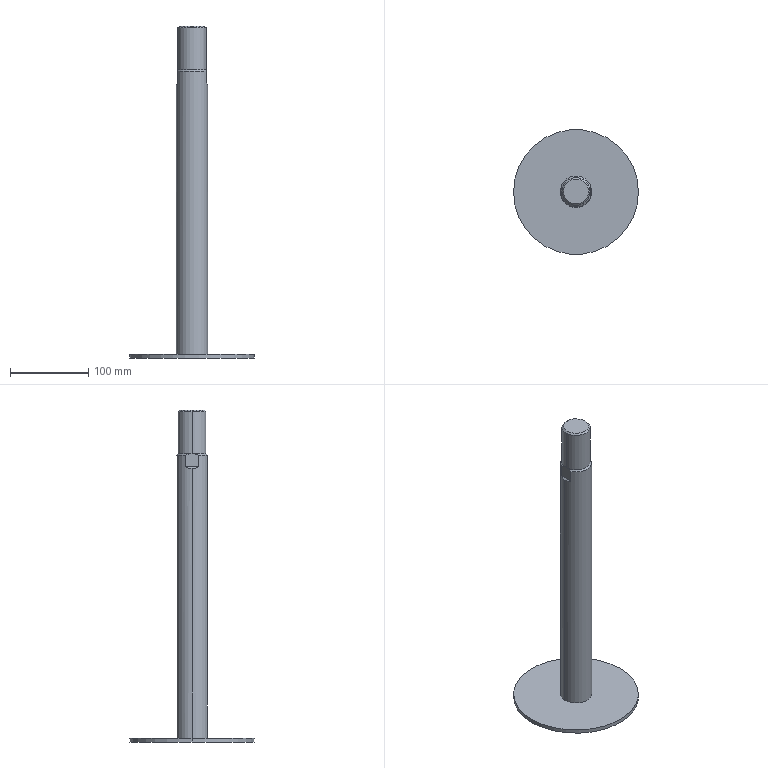Part | STEP file | CDS1FN160-250-A54Z_CS1-Rod | 1 solid | 17 faces | box 160 x 160 x 425.5 mm | volume 614336 mm3 | plane 7 | cylinder 6 | cone 4 | commonest cylinder face diameters 36 x2 40 x2 160 x2
STEP:
#1=CARTESIAN_POINT('',(0.,0.,0.));
#2=DIRECTION('',(0.,0.,1.));
#3=DIRECTION('',(1.,0.,0.));
#4=AXIS2_PLACEMENT_3D('',#1,#2,#3);
#5=CARTESIAN_POINT('',(-18.,0.,423.5));
#6=VERTEX_POINT('',#5);
#7=CARTESIAN_POINT('',(18.,0.,423.5));
#8=VERTEX_POINT('',#7);
#9=CARTESIAN_POINT('',(0.,0.,423.5));
#10=DIRECTION('',(0.,0.,-1.));
#11=DIRECTION('',(-1.,0.,0.));
#12=AXIS2_PLACEMENT_3D('',#9,#10,#11);
#13=CIRCLE('',#12,18.);
#14=CARTESIAN_POINT('',(0.,0.,0.));
#15=DIRECTION('',(0.,0.,-1.));
#16=DIRECTION('',(-1.,0.,0.));
#17=AXIS2_PLACEMENT_3D('',#14,#15,#16);
#18=CYLINDRICAL_SURFACE('',#17,18.);
#19=CARTESIAN_POINT('',(0.,-423.5));
#20=DIRECTION('',(1.,0.));
#21=VECTOR('',#20,1.);
#22=LINE('',#19,#21);
#23=(GEOMETRIC_REPRESENTATION_CONTEXT(2)PARAMETRIC_REPRESENTATION_CONTEXT()REPRESENTATION_CONTEXT('',''));
#24=DEFINITIONAL_REPRESENTATION('',(#22),#23);
#25=PCURVE('',#18,#24);
#26=CARTESIAN_POINT('',(0.,0.,425.5));
#27=DIRECTION('',(0.,0.,-1.));
#28=DIRECTION('',(-1.,0.,0.));
#29=AXIS2_PLACEMENT_3D('',#26,#27,#28);
#30=CONICAL_SURFACE('',#29,16.,0.7854);
#31=CARTESIAN_POINT('',(0.,2.));
#32=DIRECTION('',(1.,0.));
#33=VECTOR('',#32,1.);
#34=LINE('',#31,#33);
#35=(GEOMETRIC_REPRESENTATION_CONTEXT(2)PARAMETRIC_REPRESENTATION_CONTEXT()REPRESENTATION_CONTEXT('',''));
#36=DEFINITIONAL_REPRESENTATION('',(#34),#35);
#37=PCURVE('',#30,#36);
#38=SURFACE_CURVE('',#13,(#25,#37),.PCURVE_S1.);
#39=EDGE_CURVE('',#6,#8,#38,.T.);
#40=ORIENTED_EDGE('',*,*,#39,.T.);
#41=CARTESIAN_POINT('',(18.,0.,369.5));
#42=VERTEX_POINT('',#41);
#43=CARTESIAN_POINT('',(18.,0.,0.));
#44=DIRECTION('',(0.,0.,-1.));
#45=VECTOR('',#44,1.);
#46=LINE('',#43,#45);
#47=CARTESIAN_POINT('',(3.142,0.));
#48=DIRECTION('',(0.,1.));
#49=VECTOR('',#48,1.);
#50=LINE('',#47,#49);
#51=(GEOMETRIC_REPRESENTATION_CONTEXT(2)PARAMETRIC_REPRESENTATION_CONTEXT()REPRESENTATION_CONTEXT('',''));
#52=DEFINITIONAL_REPRESENTATION('',(#50),#51);
#53=PCURVE('',#18,#52);
#54=CARTESIAN_POINT('',(0.,0.,0.));
#55=DIRECTION('',(0.,0.,-1.));
#56=DIRECTION('',(-1.,0.,0.));
#57=AXIS2_PLACEMENT_3D('',#54,#55,#56);
#58=CYLINDRICAL_SURFACE('',#57,18.);
#59=CARTESIAN_POINT('',(3.142,0.));
#60=DIRECTION('',(0.,1.));
#61=VECTOR('',#60,1.);
#62=LINE('',#59,#61);
#63=(GEOMETRIC_REPRESENTATION_CONTEXT(2)PARAMETRIC_REPRESENTATION_CONTEXT()REPRESENTATION_CONTEXT('',''));
#64=DEFINITIONAL_REPRESENTATION('',(#62),#63);
#65=PCURVE('',#58,#64);
#66=SURFACE_CURVE('',#46,(#53,#65),.PCURVE_S1.);
#67=EDGE_CURVE('',#8,#42,#66,.T.);
#68=ORIENTED_EDGE('',*,*,#67,.T.);
#69=CARTESIAN_POINT('',(-18.,0.,369.5));
#70=VERTEX_POINT('',#69);
#71=CARTESIAN_POINT('',(0.,0.,369.5));
#72=DIRECTION('',(0.,0.,-1.));
#73=DIRECTION('',(-1.,0.,0.));
#74=AXIS2_PLACEMENT_3D('',#71,#72,#73);
#75=CIRCLE('',#74,18.);
#76=CARTESIAN_POINT('',(0.,-369.5));
#77=DIRECTION('',(1.,0.));
#78=VECTOR('',#77,1.);
#79=LINE('',#76,#78);
#80=(GEOMETRIC_REPRESENTATION_CONTEXT(2)PARAMETRIC_REPRESENTATION_CONTEXT()REPRESENTATION_CONTEXT('',''));
#81=DEFINITIONAL_REPRESENTATION('',(#79),#80);
#82=PCURVE('',#18,#81);
#83=CARTESIAN_POINT('',(0.,0.,369.5));
#84=DIRECTION('',(0.,0.,-1.));
#85=DIRECTION('',(-1.,0.,0.));
#86=AXIS2_PLACEMENT_3D('',#83,#84,#85);
#87=CONICAL_SURFACE('',#86,18.,0.7854);
#88=CARTESIAN_POINT('',(0.,0.));
#89=DIRECTION('',(1.,0.));
#90=VECTOR('',#89,1.);
#91=LINE('',#88,#90);
#92=(GEOMETRIC_REPRESENTATION_CONTEXT(2)PARAMETRIC_REPRESENTATION_CONTEXT()REPRESENTATION_CONTEXT('',''));
#93=DEFINITIONAL_REPRESENTATION('',(#91),#92);
#94=PCURVE('',#87,#93);
#95=SURFACE_CURVE('',#75,(#82,#94),.PCURVE_S1.);
#96=EDGE_CURVE('',#70,#42,#95,.T.);
#97=ORIENTED_EDGE('',*,*,#96,.F.);
#98=CARTESIAN_POINT('',(-18.,0.,0.));
#99=DIRECTION('',(0.,0.,-1.));
#100=VECTOR('',#99,1.);
#101=LINE('',#98,#100);
#102=CARTESIAN_POINT('',(0.,0.));
#103=DIRECTION('',(0.,1.));
#104=VECTOR('',#103,1.);
#105=LINE('',#102,#104);
#106=(GEOMETRIC_REPRESENTATION_CONTEXT(2)PARAMETRIC_REPRESENTATION_CONTEXT()REPRESENTATION_CONTEXT('',''));
#107=DEFINITIONAL_REPRESENTATION('',(#105),#106);
#108=PCURVE('',#18,#107);
#109=CARTESIAN_POINT('',(6.283,0.));
#110=DIRECTION('',(0.,1.));
#111=VECTOR('',#110,1.);
#112=LINE('',#109,#111);
#113=(GEOMETRIC_REPRESENTATION_CONTEXT(2)PARAMETRIC_REPRESENTATION_CONTEXT()REPRESENTATION_CONTEXT('',''));
#114=DEFINITIONAL_REPRESENTATION('',(#112),#113);
#115=PCURVE('',#58,#114);
#116=SURFACE_CURVE('',#101,(#108,#115),.PCURVE_S1.);
#117=EDGE_CURVE('',#6,#70,#116,.T.);
#118=ORIENTED_EDGE('',*,*,#117,.F.);
#119=EDGE_LOOP('',(#40,#68,#97,#118));
#120=FACE_BOUND('',#119,.T.);
#121=ADVANCED_FACE('',(#120),#18,.T.);
#122=CARTESIAN_POINT('',(-16.,0.,425.5));
#123=VERTEX_POINT('',#122);
#124=CARTESIAN_POINT('',(16.,0.,425.5));
#125=VERTEX_POINT('',#124);
#126=CARTESIAN_POINT('',(0.,0.,425.5));
#127=DIRECTION('',(0.,0.,-1.));
#128=DIRECTION('',(-1.,0.,0.));
#129=AXIS2_PLACEMENT_3D('',#126,#127,#128);
#130=CIRCLE('',#129,16.);
#131=CARTESIAN_POINT('',(0.,0.));
#132=DIRECTION('',(1.,0.));
#133=VECTOR('',#132,1.);
#134=LINE('',#131,#133);
#135=(GEOMETRIC_REPRESENTATION_CONTEXT(2)PARAMETRIC_REPRESENTATION_CONTEXT()REPRESENTATION_CONTEXT('',''));
#136=DEFINITIONAL_REPRESENTATION('',(#134),#135);
#137=PCURVE('',#30,#136);
#138=CARTESIAN_POINT('',(0.,0.,425.5));
#139=DIRECTION('',(0.,0.,-1.));
#140=DIRECTION('',(-1.,0.,0.));
#141=AXIS2_PLACEMENT_3D('',#138,#139,#140);
#142=PLANE('',#141);
#143=CARTESIAN_POINT('',(0.,0.));
#144=DIRECTION('',(1.,0.));
#145=AXIS2_PLACEMENT_2D('',#143,#144);
#146=CIRCLE('',#145,16.);
#147=(GEOMETRIC_REPRESENTATION_CONTEXT(2)PARAMETRIC_REPRESENTATION_CONTEXT()REPRESENTATION_CONTEXT('',''));
#148=DEFINITIONAL_REPRESENTATION('',(#146),#147);
#149=PCURVE('',#142,#148);
#150=SURFACE_CURVE('',#130,(#137,#149),.PCURVE_S1.);
#151=EDGE_CURVE('',#123,#125,#150,.T.);
#152=ORIENTED_EDGE('',*,*,#151,.T.);
#153=CARTESIAN_POINT('',(16.,0.,425.5));
#154=DIRECTION('',(0.7071,0.,-0.7071));
#155=VECTOR('',#154,1.);
#156=LINE('',#153,#155);
#157=CARTESIAN_POINT('',(3.142,0.));
#158=DIRECTION('',(0.,1.));
#159=VECTOR('',#158,1.);
#160=LINE('',#157,#159);
#161=(GEOMETRIC_REPRESENTATION_CONTEXT(2)PARAMETRIC_REPRESENTATION_CONTEXT()REPRESENTATION_CONTEXT('',''));
#162=DEFINITIONAL_REPRESENTATION('',(#160),#161);
#163=PCURVE('',#30,#162);
#164=CARTESIAN_POINT('',(0.,0.,425.5));
#165=DIRECTION('',(0.,0.,-1.));
#166=DIRECTION('',(-1.,0.,0.));
#167=AXIS2_PLACEMENT_3D('',#164,#165,#166);
#168=CONICAL_SURFACE('',#167,16.,0.7854);
#169=CARTESIAN_POINT('',(3.142,0.));
#170=DIRECTION('',(0.,1.));
#171=VECTOR('',#170,1.);
#172=LINE('',#169,#171);
#173=(GEOMETRIC_REPRESENTATION_CONTEXT(2)PARAMETRIC_REPRESENTATION_CONTEXT()REPRESENTATION_CONTEXT('',''));
#174=DEFINITIONAL_REPRESENTATION('',(#172),#173);
#175=PCURVE('',#168,#174);
#176=SURFACE_CURVE('',#156,(#163,#175),.PCURVE_S1.);
#177=EDGE_CURVE('',#125,#8,#176,.T.);
#178=ORIENTED_EDGE('',*,*,#177,.T.);
#179=ORIENTED_EDGE('',*,*,#39,.F.);
#180=CARTESIAN_POINT('',(-16.,0.,425.5));
#181=DIRECTION('',(-0.7071,0.,-0.7071));
#182=VECTOR('',#181,1.);
#183=LINE('',#180,#182);
#184=CARTESIAN_POINT('',(0.,0.));
#185=DIRECTION('',(0.,1.));
#186=VECTOR('',#185,1.);
#187=LINE('',#184,#186);
#188=(GEOMETRIC_REPRESENTATION_CONTEXT(2)PARAMETRIC_REPRESENTATION_CONTEXT()REPRESENTATION_CONTEXT('',''));
#189=DEFINITIONAL_REPRESENTATION('',(#187),#188);
#190=PCURVE('',#30,#189);
#191=CARTESIAN_POINT('',(6.283,0.));
#192=DIRECTION('',(0.,1.));
#193=VECTOR('',#192,1.);
#194=LINE('',#191,#193);
#195=(GEOMETRIC_REPRESENTATION_CONTEXT(2)PARAMETRIC_REPRESENTATION_CONTEXT()REPRESENTATION_CONTEXT('',''));
#196=DEFINITIONAL_REPRESENTATION('',(#194),#195);
#197=PCURVE('',#168,#196);
#198=SURFACE_CURVE('',#183,(#190,#197),.PCURVE_S1.);
#199=EDGE_CURVE('',#123,#6,#198,.T.);
#200=ORIENTED_EDGE('',*,*,#199,.F.);
#201=EDGE_LOOP('',(#152,#178,#179,#200));
#202=FACE_BOUND('',#201,.T.);
#203=ADVANCED_FACE('',(#202),#30,.T.);
#204=CARTESIAN_POINT('',(-80.,0.,5.));
#205=VERTEX_POINT('',#204);
#206=CARTESIAN_POINT('',(80.,0.,5.));
#207=VERTEX_POINT('',#206);
#208=CARTESIAN_POINT('',(0.,0.,5.));
#209=DIRECTION('',(0.,0.,-1.));
#210=DIRECTION('',(-1.,0.,0.));
#211=AXIS2_PLACEMENT_3D('',#208,#209,#210);
#212=CIRCLE('',#211,80.);
#213=CARTESIAN_POINT('',(0.,0.,5.));
#214=DIRECTION('',(0.,0.,-1.));
#215=DIRECTION('',(-1.,0.,0.));
#216=AXIS2_PLACEMENT_3D('',#213,#214,#215);
#217=CYLINDRICAL_SURFACE('',#216,80.);
#218=CARTESIAN_POINT('',(0.,0.));
#219=DIRECTION('',(1.,0.));
#220=VECTOR('',#219,1.);
#221=LINE('',#218,#220);
#222=(GEOMETRIC_REPRESENTATION_CONTEXT(2)PARAMETRIC_REPRESENTATION_CONTEXT()REPRESENTATION_CONTEXT('',''));
#223=DEFINITIONAL_REPRESENTATION('',(#221),#222);
#224=PCURVE('',#217,#223);
#225=CARTESIAN_POINT('',(0.,0.,5.));
#226=DIRECTION('',(0.,0.,-1.));
#227=DIRECTION('',(-1.,0.,0.));
#228=AXIS2_PLACEMENT_3D('',#225,#226,#227);
#229=PLANE('',#228);
#230=CARTESIAN_POINT('',(0.,0.));
#231=DIRECTION('',(1.,0.));
#232=AXIS2_PLACEMENT_2D('',#230,#231);
#233=CIRCLE('',#232,80.);
#234=(GEOMETRIC_REPRESENTATION_CONTEXT(2)PARAMETRIC_REPRESENTATION_CONTEXT()REPRESENTATION_CONTEXT('',''));
#235=DEFINITIONAL_REPRESENTATION('',(#233),#234);
#236=PCURVE('',#229,#235);
#237=SURFACE_CURVE('',#212,(#224,#236),.PCURVE_S1.);
#238=EDGE_CURVE('',#205,#207,#237,.T.);
#239=ORIENTED_EDGE('',*,*,#238,.T.);
#240=CARTESIAN_POINT('',(80.,0.,0.));
#241=VERTEX_POINT('',#240);
#242=CARTESIAN_POINT('',(80.,0.,5.));
#243=DIRECTION('',(0.,0.,-1.));
#244=VECTOR('',#243,1.);
#245=LINE('',#242,#244);
#246=CARTESIAN_POINT('',(3.142,0.));
#247=DIRECTION('',(0.,1.));
#248=VECTOR('',#247,1.);
#249=LINE('',#246,#248);
#250=(GEOMETRIC_REPRESENTATION_CONTEXT(2)PARAMETRIC_REPRESENTATION_CONTEXT()REPRESENTATION_CONTEXT('',''));
#251=DEFINITIONAL_REPRESENTATION('',(#249),#250);
#252=PCURVE('',#217,#251);
#253=CARTESIAN_POINT('',(0.,0.,5.));
#254=DIRECTION('',(0.,0.,-1.));
#255=DIRECTION('',(-1.,0.,0.));
#256=AXIS2_PLACEMENT_3D('',#253,#254,#255);
#257=CYLINDRICAL_SURFACE('',#256,80.);
#258=CARTESIAN_POINT('',(3.142,0.));
#259=DIRECTION('',(0.,1.));
#260=VECTOR('',#259,1.);
#261=LINE('',#258,#260);
#262=(GEOMETRIC_REPRESENTATION_CONTEXT(2)PARAMETRIC_REPRESENTATION_CONTEXT()REPRESENTATION_CONTEXT('',''));
#263=DEFINITIONAL_REPRESENTATION('',(#261),#262);
#264=PCURVE('',#257,#263);
#265=SURFACE_CURVE('',#245,(#252,#264),.PCURVE_S1.);
#266=EDGE_CURVE('',#207,#241,#265,.T.);
#267=ORIENTED_EDGE('',*,*,#266,.T.);
#268=CARTESIAN_POINT('',(-80.,0.,0.));
#269=VERTEX_POINT('',#268);
#270=CARTESIAN_POINT('',(0.,0.,0.));
#271=DIRECTION('',(0.,0.,-1.));
#272=DIRECTION('',(-1.,0.,0.));
#273=AXIS2_PLACEMENT_3D('',#270,#271,#272);
#274=CIRCLE('',#273,80.);
#275=CARTESIAN_POINT('',(0.,5.));
#276=DIRECTION('',(1.,0.));
#277=VECTOR('',#276,1.);
#278=LINE('',#275,#277);
#279=(GEOMETRIC_REPRESENTATION_CONTEXT(2)PARAMETRIC_REPRESENTATION_CONTEXT()REPRESENTATION_CONTEXT('',''));
#280=DEFINITIONAL_REPRESENTATION('',(#278),#279);
#281=PCURVE('',#217,#280);
#282=CARTESIAN_POINT('',(0.,0.,0.));
#283=DIRECTION('',(0.,0.,1.));
#284=DIRECTION('',(1.,0.,0.));
#285=AXIS2_PLACEMENT_3D('',#282,#283,#284);
#286=PLANE('',#285);
#287=CARTESIAN_POINT('',(-80.,0.));
#288=CARTESIAN_POINT('',(-80.,138.564));
#289=CARTESIAN_POINT('',(40.,69.282));
#290=CARTESIAN_POINT('',(160.,0.));
#291=CARTESIAN_POINT('',(40.,-69.282));
#292=CARTESIAN_POINT('',(-80.,-138.564));
#293=CARTESIAN_POINT('',(-80.,0.));
#294=(BOUNDED_CURVE()B_SPLINE_CURVE(2,(#287,#288,#289,#290,#291,#292,#293),.UNSPECIFIED.,.T.,.F.)B_SPLINE_CURVE_WITH_KNOTS((1,2,2,2,2,1),(-2.094,0.,2.094,4.189,6.283,8.378),.UNSPECIFIED.)CURVE()GEOMETRIC_REPRESENTATION_ITEM()RATIONAL_B_SPLINE_CURVE((1.,0.5,1.,0.5,1.,0.5,1.))REPRESENTATION_ITEM(''));
#295=(GEOMETRIC_REPRESENTATION_CONTEXT(2)PARAMETRIC_REPRESENTATION_CONTEXT()REPRESENTATION_CONTEXT('',''));
#296=DEFINITIONAL_REPRESENTATION('',(#294),#295);
#297=PCURVE('',#286,#296);
#298=SURFACE_CURVE('',#274,(#281,#297),.PCURVE_S1.);
#299=EDGE_CURVE('',#269,#241,#298,.T.);
#300=ORIENTED_EDGE('',*,*,#299,.F.);
#301=CARTESIAN_POINT('',(-80.,0.,5.));
#302=DIRECTION('',(0.,0.,-1.));
#303=VECTOR('',#302,1.);
#304=LINE('',#301,#303);
#305=CARTESIAN_POINT('',(0.,0.));
#306=DIRECTION('',(0.,1.));
#307=VECTOR('',#306,1.);
#308=LINE('',#305,#307);
#309=(GEOMETRIC_REPRESENTATION_CONTEXT(2)PARAMETRIC_REPRESENTATION_CONTEXT()REPRESENTATION_CONTEXT('',''));
#310=DEFINITIONAL_REPRESENTATION('',(#308),#309);
#311=PCURVE('',#217,#310);
#312=CARTESIAN_POINT('',(6.283,0.));
#313=DIRECTION('',(0.,1.));
#314=VECTOR('',#313,1.);
#315=LINE('',#312,#314);
#316=(GEOMETRIC_REPRESENTATION_CONTEXT(2)PARAMETRIC_REPRESENTATION_CONTEXT()REPRESENTATION_CONTEXT('',''));
#317=DEFINITIONAL_REPRESENTATION('',(#315),#316);
#318=PCURVE('',#257,#317);
#319=SURFACE_CURVE('',#304,(#311,#318),.PCURVE_S1.);
#320=EDGE_CURVE('',#205,#269,#319,.T.);
#321=ORIENTED_EDGE('',*,*,#320,.F.);
#322=EDGE_LOOP('',(#239,#267,#300,#321));
#323=FACE_BOUND('',#322,.T.);
#324=ADVANCED_FACE('',(#323),#217,.T.);
#325=CARTESIAN_POINT('',(18.,8.718,352.5));
#326=VERTEX_POINT('',#325);
#327=CARTESIAN_POINT('',(20.,0.,350.5));
#328=VERTEX_POINT('',#327);
#329=CARTESIAN_POINT('',(18.,8.718,352.5));
#330=CARTESIAN_POINT('',(19.322,5.988,351.178));
#331=CARTESIAN_POINT('',(20.,3.033,350.5));
#332=CARTESIAN_POINT('',(20.,0.,350.5));
#333=(BOUNDED_CURVE()B_SPLINE_CURVE(3,(#329,#330,#331,#332),.UNSPECIFIED.,.F.,.F.)B_SPLINE_CURVE_WITH_KNOTS((4,4),(5.832,6.283),.PIECEWISE_BEZIER_KNOTS.)CURVE()GEOMETRIC_REPRESENTATION_ITEM()RATIONAL_B_SPLINE_CURVE((1.,0.9831,0.9831,1.))REPRESENTATION_ITEM(''));
#334=CARTESIAN_POINT('',(0.,0.,482.069));
#335=DIRECTION('',(0.,0.,-1.));
#336=DIRECTION('',(-1.,0.,0.));
#337=AXIS2_PLACEMENT_3D('',#334,#335,#336);
#338=CYLINDRICAL_SURFACE('',#337,20.);
#339=CARTESIAN_POINT('',(2.691,129.569));
#340=CARTESIAN_POINT('',(2.697,129.628));
#341=CARTESIAN_POINT('',(2.711,129.743));
#342=CARTESIAN_POINT('',(2.731,129.91));
#343=CARTESIAN_POINT('',(2.752,130.069));
#344=CARTESIAN_POINT('',(2.772,130.221));
#345=CARTESIAN_POINT('',(2.793,130.365));
#346=CARTESIAN_POINT('',(2.813,130.501));
#347=CARTESIAN_POINT('',(2.834,130.63));
#348=CARTESIAN_POINT('',(2.854,130.75));
#349=CARTESIAN_POINT('',(2.875,130.863));
#350=CARTESIAN_POINT('',(2.895,130.967));
#351=CARTESIAN_POINT('',(2.916,131.064));
#352=CARTESIAN_POINT('',(2.937,131.151));
#353=CARTESIAN_POINT('',(2.957,131.231));
#354=CARTESIAN_POINT('',(2.978,131.302));
#355=CARTESIAN_POINT('',(2.998,131.365));
#356=CARTESIAN_POINT('',(3.019,131.42));
#357=CARTESIAN_POINT('',(3.039,131.466));
#358=CARTESIAN_POINT('',(3.06,131.503));
#359=CARTESIAN_POINT('',(3.08,131.533));
#360=CARTESIAN_POINT('',(3.101,131.553));
#361=CARTESIAN_POINT('',(3.121,131.566));
#362=CARTESIAN_POINT('',(3.135,131.569));
#363=CARTESIAN_POINT('',(3.142,131.569));
#364=B_SPLINE_CURVE_WITH_KNOTS('',3,(#339,#340,#341,#342,#343,#344,#345,#346,#347,#348,#349,#350,#351,#352,#353,#354,#355,#356,#357,#358,#359,#360,#361,#362,#363),.UNSPECIFIED.,.F.,.F.,(4,1,1,1,1,1,1,1,1,1,1,1,1,1,1,1,1,1,1,1,1,1,4),(5.832,5.853,5.873,5.894,5.914,5.935,5.955,5.976,5.996,6.017,6.037,6.058,6.078,6.099,6.119,6.14,6.16,6.181,6.201,6.222,6.242,6.263,6.283),.QUASI_UNIFORM_KNOTS.);
#365=(GEOMETRIC_REPRESENTATION_CONTEXT(2)PARAMETRIC_REPRESENTATION_CONTEXT()REPRESENTATION_CONTEXT('',''));
#366=DEFINITIONAL_REPRESENTATION('',(#364),#365);
#367=PCURVE('',#338,#366);
#368=CARTESIAN_POINT('',(20.,-80.,350.5));
#369=DIRECTION('',(-0.7071,0.,-0.7071));
#370=DIRECTION('',(-0.7071,0.,0.7071));
#371=AXIS2_PLACEMENT_3D('',#368,#369,#370);
#372=PLANE('',#371);
#373=CARTESIAN_POINT('',(2.828,88.718));
#374=CARTESIAN_POINT('',(0.959,85.988));
#375=CARTESIAN_POINT('',(0.,83.033));
#376=CARTESIAN_POINT('',(0.,80.));
#377=(BOUNDED_CURVE()B_SPLINE_CURVE(3,(#373,#374,#375,#376),.UNSPECIFIED.,.F.,.F.)B_SPLINE_CURVE_WITH_KNOTS((4,4),(5.832,6.283),.PIECEWISE_BEZIER_KNOTS.)CURVE()GEOMETRIC_REPRESENTATION_ITEM()RATIONAL_B_SPLINE_CURVE((1.,0.9831,0.9831,1.))REPRESENTATION_ITEM(''));
#378=(GEOMETRIC_REPRESENTATION_CONTEXT(2)PARAMETRIC_REPRESENTATION_CONTEXT()REPRESENTATION_CONTEXT('',''));
#379=DEFINITIONAL_REPRESENTATION('',(#377),#378);
#380=PCURVE('',#372,#379);
#381=SURFACE_CURVE('',#333,(#367,#380),.PCURVE_S1.);
#382=EDGE_CURVE('',#326,#328,#381,.T.);
#383=ORIENTED_EDGE('',*,*,#382,.T.);
#384=CARTESIAN_POINT('',(20.,0.,5.));
#385=VERTEX_POINT('',#384);
#386=CARTESIAN_POINT('',(20.,0.,482.069));
#387=DIRECTION('',(0.,0.,-1.));
#388=VECTOR('',#387,1.);
#389=LINE('',#386,#388);
#390=CARTESIAN_POINT('',(3.142,0.));
#391=DIRECTION('',(0.,1.));
#392=VECTOR('',#391,1.);
#393=LINE('',#390,#392);
#394=(GEOMETRIC_REPRESENTATION_CONTEXT(2)PARAMETRIC_REPRESENTATION_CONTEXT()REPRESENTATION_CONTEXT('',''));
#395=DEFINITIONAL_REPRESENTATION('',(#393),#394);
#396=PCURVE('',#338,#395);
#397=CARTESIAN_POINT('',(0.,0.,482.069));
#398=DIRECTION('',(0.,0.,-1.));
#399=DIRECTION('',(-1.,0.,0.));
#400=AXIS2_PLACEMENT_3D('',#397,#398,#399);
#401=CYLINDRICAL_SURFACE('',#400,20.);
#402=CARTESIAN_POINT('',(3.142,0.));
#403=DIRECTION('',(0.,1.));
#404=VECTOR('',#403,1.);
#405=LINE('',#402,#404);
#406=(GEOMETRIC_REPRESENTATION_CONTEXT(2)PARAMETRIC_REPRESENTATION_CONTEXT()REPRESENTATION_CONTEXT('',''));
#407=DEFINITIONAL_REPRESENTATION('',(#405),#406);
#408=PCURVE('',#401,#407);
#409=SURFACE_CURVE('',#389,(#396,#408),.PCURVE_S1.);
#410=EDGE_CURVE('',#328,#385,#409,.T.);
#411=ORIENTED_EDGE('',*,*,#410,.T.);
#412=CARTESIAN_POINT('',(-20.,0.,5.));
#413=VERTEX_POINT('',#412);
#414=CARTESIAN_POINT('',(0.,0.,5.));
#415=DIRECTION('',(0.,0.,-1.));
#416=DIRECTION('',(-1.,0.,0.));
#417=AXIS2_PLACEMENT_3D('',#414,#415,#416);
#418=CIRCLE('',#417,20.);
#419=CARTESIAN_POINT('',(0.,477.069));
#420=DIRECTION('',(1.,0.));
#421=VECTOR('',#420,1.);
#422=LINE('',#419,#421);
#423=(GEOMETRIC_REPRESENTATION_CONTEXT(2)PARAMETRIC_REPRESENTATION_CONTEXT()REPRESENTATION_CONTEXT('',''));
#424=DEFINITIONAL_REPRESENTATION('',(#422),#423);
#425=PCURVE('',#338,#424);
#426=CARTESIAN_POINT('',(0.,0.));
#427=DIRECTION('',(1.,0.));
#428=AXIS2_PLACEMENT_2D('',#426,#427);
#429=CIRCLE('',#428,20.);
#430=(GEOMETRIC_REPRESENTATION_CONTEXT(2)PARAMETRIC_REPRESENTATION_CONTEXT()REPRESENTATION_CONTEXT('',''));
#431=DEFINITIONAL_REPRESENTATION('',(#429),#430);
#432=PCURVE('',#229,#431);
#433=SURFACE_CURVE('',#418,(#425,#432),.PCURVE_S1.);
#434=EDGE_CURVE('',#413,#385,#433,.T.);
#435=ORIENTED_EDGE('',*,*,#434,.F.);
#436=CARTESIAN_POINT('',(-20.,0.,350.5));
#437=VERTEX_POINT('',#436);
#438=CARTESIAN_POINT('',(-20.,0.,482.069));
#439=DIRECTION('',(0.,0.,-1.));
#440=VECTOR('',#439,1.);
#441=LINE('',#438,#440);
#442=CARTESIAN_POINT('',(0.,0.));
#443=DIRECTION('',(0.,1.));
#444=VECTOR('',#443,1.);
#445=LINE('',#442,#444);
#446=(GEOMETRIC_REPRESENTATION_CONTEXT(2)PARAMETRIC_REPRESENTATION_CONTEXT()REPRESENTATION_CONTEXT('',''));
#447=DEFINITIONAL_REPRESENTATION('',(#445),#446);
#448=PCURVE('',#338,#447);
#449=CARTESIAN_POINT('',(6.283,0.));
#450=DIRECTION('',(0.,1.));
#451=VECTOR('',#450,1.);
#452=LINE('',#449,#451);
#453=(GEOMETRIC_REPRESENTATION_CONTEXT(2)PARAMETRIC_REPRESENTATION_CONTEXT()REPRESENTATION_CONTEXT('',''));
#454=DEFINITIONAL_REPRESENTATION('',(#452),#453);
#455=PCURVE('',#401,#454);
#456=SURFACE_CURVE('',#441,(#448,#455),.PCURVE_S1.);
#457=EDGE_CURVE('',#437,#413,#456,.T.);
#458=ORIENTED_EDGE('',*,*,#457,.F.);
#459=CARTESIAN_POINT('',(-18.,8.718,352.5));
#460=VERTEX_POINT('',#459);
#461=CARTESIAN_POINT('',(-20.,0.,350.5));
#462=CARTESIAN_POINT('',(-20.,3.033,350.5));
#463=CARTESIAN_POINT('',(-19.322,5.988,351.178));
#464=CARTESIAN_POINT('',(-18.,8.718,352.5));
#465=(BOUNDED_CURVE()B_SPLINE_CURVE(3,(#461,#462,#463,#464),.UNSPECIFIED.,.F.,.F.)B_SPLINE_CURVE_WITH_KNOTS((4,4),(0.,0.451),.PIECEWISE_BEZIER_KNOTS.)CURVE()GEOMETRIC_REPRESENTATION_ITEM()RATIONAL_B_SPLINE_CURVE((1.,0.9831,0.9831,1.))REPRESENTATION_ITEM(''));
#466=CARTESIAN_POINT('',(0.,131.569));
#467=CARTESIAN_POINT('',(0.006776,131.569));
#468=CARTESIAN_POINT('',(0.02034,131.566));
#469=CARTESIAN_POINT('',(0.04074,131.553));
#470=CARTESIAN_POINT('',(0.06117,131.533));
#471=CARTESIAN_POINT('',(0.08164,131.503));
#472=CARTESIAN_POINT('',(0.1021,131.466));
#473=CARTESIAN_POINT('',(0.1227,131.42));
#474=CARTESIAN_POINT('',(0.1432,131.365));
#475=CARTESIAN_POINT('',(0.1638,131.302));
#476=CARTESIAN_POINT('',(0.1843,131.231));
#477=CARTESIAN_POINT('',(0.2049,131.151));
#478=CARTESIAN_POINT('',(0.2255,131.064));
#479=CARTESIAN_POINT('',(0.2461,130.967));
#480=CARTESIAN_POINT('',(0.2667,130.863));
#481=CARTESIAN_POINT('',(0.2873,130.75));
#482=CARTESIAN_POINT('',(0.3078,130.63));
#483=CARTESIAN_POINT('',(0.3284,130.501));
#484=CARTESIAN_POINT('',(0.3489,130.365));
#485=CARTESIAN_POINT('',(0.3694,130.221));
#486=CARTESIAN_POINT('',(0.3899,130.069));
#487=CARTESIAN_POINT('',(0.4103,129.91));
#488=CARTESIAN_POINT('',(0.4307,129.743));
#489=CARTESIAN_POINT('',(0.4443,129.628));
#490=CARTESIAN_POINT('',(0.451,129.569));
#491=B_SPLINE_CURVE_WITH_KNOTS('',3,(#466,#467,#468,#469,#470,#471,#472,#473,#474,#475,#476,#477,#478,#479,#480,#481,#482,#483,#484,#485,#486,#487,#488,#489,#490),.UNSPECIFIED.,.F.,.F.,(4,1,1,1,1,1,1,1,1,1,1,1,1,1,1,1,1,1,1,1,1,1,4),(0.,0.0205,0.041,0.0615,0.082,0.1025,0.123,0.1435,0.164,0.1845,0.205,0.2255,0.246,0.2665,0.287,0.3075,0.328,0.3485,0.369,0.3895,0.41,0.4305,0.451),.QUASI_UNIFORM_KNOTS.);
#492=(GEOMETRIC_REPRESENTATION_CONTEXT(2)PARAMETRIC_REPRESENTATION_CONTEXT()REPRESENTATION_CONTEXT('',''));
#493=DEFINITIONAL_REPRESENTATION('',(#491),#492);
#494=PCURVE('',#338,#493);
#495=CARTESIAN_POINT('',(-20.,-80.,350.5));
#496=DIRECTION('',(0.7071,0.,-0.7071));
#497=DIRECTION('',(-0.7071,0.,-0.7071));
#498=AXIS2_PLACEMENT_3D('',#495,#496,#497);
#499=PLANE('',#498);
#500=CARTESIAN_POINT('',(0.,80.));
#501=CARTESIAN_POINT('',(0.,83.033));
#502=CARTESIAN_POINT('',(-0.959,85.988));
#503=CARTESIAN_POINT('',(-2.828,88.718));
#504=(BOUNDED_CURVE()B_SPLINE_CURVE(3,(#500,#501,#502,#503),.UNSPECIFIED.,.F.,.F.)B_SPLINE_CURVE_WITH_KNOTS((4,4),(0.,0.451),.PIECEWISE_BEZIER_KNOTS.)CURVE()GEOMETRIC_REPRESENTATION_ITEM()RATIONAL_B_SPLINE_CURVE((1.,0.9831,0.9831,1.))REPRESENTATION_ITEM(''));
#505=(GEOMETRIC_REPRESENTATION_CONTEXT(2)PARAMETRIC_REPRESENTATION_CONTEXT()REPRESENTATION_CONTEXT('',''));
#506=DEFINITIONAL_REPRESENTATION('',(#504),#505);
#507=PCURVE('',#499,#506);
#508=SURFACE_CURVE('',#465,(#494,#507),.PCURVE_S1.);
#509=EDGE_CURVE('',#437,#460,#508,.T.);
#510=ORIENTED_EDGE('',*,*,#509,.T.);
#511=CARTESIAN_POINT('',(-18.,8.718,367.5));
#512=VERTEX_POINT('',#511);
#513=CARTESIAN_POINT('',(-18.,8.718,482.069));
#514=DIRECTION('',(0.,0.,1.));
#515=VECTOR('',#514,1.);
#516=LINE('',#513,#515);
#517=CARTESIAN_POINT('',(0.451,0.));
#518=DIRECTION('',(0.,-1.));
#519=VECTOR('',#518,1.);
#520=LINE('',#517,#519);
#521=(GEOMETRIC_REPRESENTATION_CONTEXT(2)PARAMETRIC_REPRESENTATION_CONTEXT()REPRESENTATION_CONTEXT('',''));
#522=DEFINITIONAL_REPRESENTATION('',(#520),#521);
#523=PCURVE('',#338,#522);
#524=CARTESIAN_POINT('',(-18.,-80.,352.5));
#525=DIRECTION('',(1.,0.,0.));
#526=DIRECTION('',(0.,0.,-1.));
#527=AXIS2_PLACEMENT_3D('',#524,#525,#526);
#528=PLANE('',#527);
#529=CARTESIAN_POINT('',(-129.569,88.718));
#530=DIRECTION('',(-1.,0.));
#531=VECTOR('',#530,1.);
#532=LINE('',#529,#531);
#533=(GEOMETRIC_REPRESENTATION_CONTEXT(2)PARAMETRIC_REPRESENTATION_CONTEXT()REPRESENTATION_CONTEXT('',''));
#534=DEFINITIONAL_REPRESENTATION('',(#532),#533);
#535=PCURVE('',#528,#534);
#536=SURFACE_CURVE('',#516,(#523,#535),.PCURVE_S1.);
#537=EDGE_CURVE('',#460,#512,#536,.T.);
#538=ORIENTED_EDGE('',*,*,#537,.T.);
#539=CARTESIAN_POINT('',(18.,8.718,367.5));
#540=VERTEX_POINT('',#539);
#541=CARTESIAN_POINT('',(0.,0.,367.5));
#542=DIRECTION('',(0.,0.,-1.));
#543=DIRECTION('',(-1.,0.,0.));
#544=AXIS2_PLACEMENT_3D('',#541,#542,#543);
#545=CIRCLE('',#544,20.);
#546=CARTESIAN_POINT('',(0.,114.569));
#547=DIRECTION('',(1.,0.));
#548=VECTOR('',#547,1.);
#549=LINE('',#546,#548);
#550=(GEOMETRIC_REPRESENTATION_CONTEXT(2)PARAMETRIC_REPRESENTATION_CONTEXT()REPRESENTATION_CONTEXT('',''));
#551=DEFINITIONAL_REPRESENTATION('',(#549),#550);
#552=PCURVE('',#338,#551);
#553=CARTESIAN_POINT('',(0.,2.));
#554=DIRECTION('',(1.,0.));
#555=VECTOR('',#554,1.);
#556=LINE('',#553,#555);
#557=(GEOMETRIC_REPRESENTATION_CONTEXT(2)PARAMETRIC_REPRESENTATION_CONTEXT()REPRESENTATION_CONTEXT('',''));
#558=DEFINITIONAL_REPRESENTATION('',(#556),#557);
#559=PCURVE('',#87,#558);
#560=SURFACE_CURVE('',#545,(#552,#559),.PCURVE_S1.);
#561=EDGE_CURVE('',#512,#540,#560,.T.);
#562=ORIENTED_EDGE('',*,*,#561,.T.);
#563=CARTESIAN_POINT('',(18.,8.718,482.069));
#564=DIRECTION('',(0.,0.,-1.));
#565=VECTOR('',#564,1.);
#566=LINE('',#563,#565);
#567=CARTESIAN_POINT('',(2.691,0.));
#568=DIRECTION('',(0.,1.));
#569=VECTOR('',#568,1.);
#570=LINE('',#567,#569);
#571=(GEOMETRIC_REPRESENTATION_CONTEXT(2)PARAMETRIC_REPRESENTATION_CONTEXT()REPRESENTATION_CONTEXT('',''));
#572=DEFINITIONAL_REPRESENTATION('',(#570),#571);
#573=PCURVE('',#338,#572);
#574=CARTESIAN_POINT('',(18.,-80.,352.5));
#575=DIRECTION('',(-1.,0.,0.));
#576=DIRECTION('',(0.,0.,1.));
#577=AXIS2_PLACEMENT_3D('',#574,#575,#576);
#578=PLANE('',#577);
#579=CARTESIAN_POINT('',(129.569,88.718));
#580=DIRECTION('',(-1.,0.));
#581=VECTOR('',#580,1.);
#582=LINE('',#579,#581);
#583=(GEOMETRIC_REPRESENTATION_CONTEXT(2)PARAMETRIC_REPRESENTATION_CONTEXT()REPRESENTATION_CONTEXT('',''));
#584=DEFINITIONAL_REPRESENTATION('',(#582),#583);
#585=PCURVE('',#578,#584);
#586=SURFACE_CURVE('',#566,(#573,#585),.PCURVE_S1.);
#587=EDGE_CURVE('',#540,#326,#586,.T.);
#588=ORIENTED_EDGE('',*,*,#587,.T.);
#589=EDGE_LOOP('',(#383,#411,#435,#458,#510,#538,#562,#588));
#590=FACE_BOUND('',#589,.T.);
#591=ADVANCED_FACE('',(#590),#338,.T.);
#592=ORIENTED_EDGE('',*,*,#561,.F.);
#593=CARTESIAN_POINT('',(-18.,8.718,367.5));
#594=CARTESIAN_POINT('',(-18.,8.033,367.799));
#595=CARTESIAN_POINT('',(-18.,7.333,368.075));
#596=CARTESIAN_POINT('',(-18.,5.906,368.568));
#597=CARTESIAN_POINT('',(-18.,5.187,368.781));
#598=CARTESIAN_POINT('',(-18.,3.732,369.131));
#599=CARTESIAN_POINT('',(-18.,2.997,369.267));
#600=CARTESIAN_POINT('',(-18.,1.883,369.406));
#601=CARTESIAN_POINT('',(-18.,1.509,369.441));
#602=CARTESIAN_POINT('',(-18.,0.7572,369.488));
#603=CARTESIAN_POINT('',(-18.,0.3777,369.5));
#604=CARTESIAN_POINT('',(-18.,0.,369.5));
#605=B_SPLINE_CURVE_WITH_KNOTS('',3,(#593,#594,#595,#596,#597,#598,#599,#600,#601,#602,#603,#604),.UNSPECIFIED.,.F.,.F.,(4,2,2,2,2,4),(0.01306,0.01529,0.01752,0.01975,0.02086,0.02197),.UNSPECIFIED.);
#606=CARTESIAN_POINT('',(0.451,2.));
#607=CARTESIAN_POINT('',(0.4454,1.946));
#608=CARTESIAN_POINT('',(0.4341,1.839));
#609=CARTESIAN_POINT('',(0.4167,1.683));
#610=CARTESIAN_POINT('',(0.3988,1.532));
#611=CARTESIAN_POINT('',(0.3806,1.386));
#612=CARTESIAN_POINT('',(0.362,1.246));
#613=CARTESIAN_POINT('',(0.3429,1.111));
#614=CARTESIAN_POINT('',(0.3235,0.9835));
#615=CARTESIAN_POINT('',(0.3038,0.8626));
#616=CARTESIAN_POINT('',(0.2838,0.7487));
#617=CARTESIAN_POINT('',(0.2635,0.6421));
#618=CARTESIAN_POINT('',(0.2429,0.5429));
#619=CARTESIAN_POINT('',(0.222,0.4513));
#620=CARTESIAN_POINT('',(0.2008,0.3676));
#621=CARTESIAN_POINT('',(0.1793,0.2919));
#622=CARTESIAN_POINT('',(0.1576,0.2245));
#623=CARTESIAN_POINT('',(0.1357,0.1654));
#624=CARTESIAN_POINT('',(0.1135,0.1151));
#625=CARTESIAN_POINT('',(0.09113,0.07346));
#626=CARTESIAN_POINT('',(0.06856,0.04083));
#627=CARTESIAN_POINT('',(0.04582,0.01734));
#628=CARTESIAN_POINT('',(0.02292,0.003165));
#629=CARTESIAN_POINT('',(0.007631,-0.000006235));
#630=CARTESIAN_POINT('',(0.,0.));
#631=B_SPLINE_CURVE_WITH_KNOTS('',3,(#606,#607,#608,#609,#610,#611,#612,#613,#614,#615,#616,#617,#618,#619,#620,#621,#622,#623,#624,#625,#626,#627,#628,#629,#630),.UNSPECIFIED.,.F.,.F.,(4,1,1,1,1,1,1,1,1,1,1,1,1,1,1,1,1,1,1,1,1,1,4),(0.01306,0.01347,0.01387,0.01428,0.01468,0.01509,0.01549,0.0159,0.0163,0.01671,0.01711,0.01752,0.01792,0.01833,0.01873,0.01914,0.01954,0.01995,0.02035,0.02076,0.02116,0.02157,0.02197),.QUASI_UNIFORM_KNOTS.);
#632=(GEOMETRIC_REPRESENTATION_CONTEXT(2)PARAMETRIC_REPRESENTATION_CONTEXT()REPRESENTATION_CONTEXT('',''));
#633=DEFINITIONAL_REPRESENTATION('',(#631),#632);
#634=PCURVE('',#87,#633);
#635=CARTESIAN_POINT('',(-15.,88.718));
#636=CARTESIAN_POINT('',(-15.299,88.033));
#637=CARTESIAN_POINT('',(-15.575,87.333));
#638=CARTESIAN_POINT('',(-16.068,85.906));
#639=CARTESIAN_POINT('',(-16.281,85.187));
#640=CARTESIAN_POINT('',(-16.631,83.732));
#641=CARTESIAN_POINT('',(-16.767,82.997));
#642=CARTESIAN_POINT('',(-16.906,81.883));
#643=CARTESIAN_POINT('',(-16.941,81.509));
#644=CARTESIAN_POINT('',(-16.988,80.757));
#645=CARTESIAN_POINT('',(-17.,80.378));
#646=CARTESIAN_POINT('',(-17.,80.));
#647=B_SPLINE_CURVE_WITH_KNOTS('',3,(#635,#636,#637,#638,#639,#640,#641,#642,#643,#644,#645,#646),.UNSPECIFIED.,.F.,.F.,(4,2,2,2,2,4),(0.01306,0.01529,0.01752,0.01975,0.02086,0.02197),.UNSPECIFIED.);
#648=(GEOMETRIC_REPRESENTATION_CONTEXT(2)PARAMETRIC_REPRESENTATION_CONTEXT()REPRESENTATION_CONTEXT('',''));
#649=DEFINITIONAL_REPRESENTATION('',(#647),#648);
#650=PCURVE('',#528,#649);
#651=SURFACE_CURVE('',#605,(#634,#650),.PCURVE_S1.);
#652=EDGE_CURVE('',#512,#70,#651,.T.);
#653=ORIENTED_EDGE('',*,*,#652,.T.);
#654=ORIENTED_EDGE('',*,*,#96,.T.);
#655=CARTESIAN_POINT('',(18.,0.,369.5));
#656=CARTESIAN_POINT('',(18.,0.3777,369.5));
#657=CARTESIAN_POINT('',(18.,0.7572,369.488));
#658=CARTESIAN_POINT('',(18.,1.509,369.441));
#659=CARTESIAN_POINT('',(18.,1.883,369.406));
#660=CARTESIAN_POINT('',(18.,2.997,369.267));
#661=CARTESIAN_POINT('',(18.,3.732,369.131));
#662=CARTESIAN_POINT('',(18.,5.187,368.781));
#663=CARTESIAN_POINT('',(18.,5.906,368.568));
#664=CARTESIAN_POINT('',(18.,7.333,368.075));
#665=CARTESIAN_POINT('',(18.,8.033,367.799));
#666=CARTESIAN_POINT('',(18.,8.718,367.5));
#667=B_SPLINE_CURVE_WITH_KNOTS('',3,(#655,#656,#657,#658,#659,#660,#661,#662,#663,#664,#665,#666),.UNSPECIFIED.,.F.,.F.,(4,2,2,2,2,4),(0.01468,0.0158,0.01692,0.01916,0.0214,0.02364),.UNSPECIFIED.);
#668=CARTESIAN_POINT('',(3.142,0.));
#669=CARTESIAN_POINT('',(3.134,-0.000006235));
#670=CARTESIAN_POINT('',(3.119,0.003165));
#671=CARTESIAN_POINT('',(3.096,0.01734));
#672=CARTESIAN_POINT('',(3.073,0.04083));
#673=CARTESIAN_POINT('',(3.05,0.07346));
#674=CARTESIAN_POINT('',(3.028,0.1151));
#675=CARTESIAN_POINT('',(3.006,0.1654));
#676=CARTESIAN_POINT('',(2.984,0.2245));
#677=CARTESIAN_POINT('',(2.962,0.2919));
#678=CARTESIAN_POINT('',(2.941,0.3676));
#679=CARTESIAN_POINT('',(2.92,0.4513));
#680=CARTESIAN_POINT('',(2.899,0.5429));
#681=CARTESIAN_POINT('',(2.878,0.6421));
#682=CARTESIAN_POINT('',(2.858,0.7487));
#683=CARTESIAN_POINT('',(2.838,0.8626));
#684=CARTESIAN_POINT('',(2.818,0.9835));
#685=CARTESIAN_POINT('',(2.799,1.111));
#686=CARTESIAN_POINT('',(2.78,1.246));
#687=CARTESIAN_POINT('',(2.761,1.386));
#688=CARTESIAN_POINT('',(2.743,1.532));
#689=CARTESIAN_POINT('',(2.725,1.683));
#690=CARTESIAN_POINT('',(2.708,1.839));
#691=CARTESIAN_POINT('',(2.696,1.946));
#692=CARTESIAN_POINT('',(2.691,2.));
#693=B_SPLINE_CURVE_WITH_KNOTS('',3,(#668,#669,#670,#671,#672,#673,#674,#675,#676,#677,#678,#679,#680,#681,#682,#683,#684,#685,#686,#687,#688,#689,#690,#691,#692),.UNSPECIFIED.,.F.,.F.,(4,1,1,1,1,1,1,1,1,1,1,1,1,1,1,1,1,1,1,1,1,1,4),(0.01468,0.01508,0.01549,0.0159,0.0163,0.01671,0.01712,0.01753,0.01793,0.01834,0.01875,0.01916,0.01956,0.01997,0.02038,0.02078,0.02119,0.0216,0.02201,0.02241,0.02282,0.02323,0.02364),.QUASI_UNIFORM_KNOTS.);
#694=(GEOMETRIC_REPRESENTATION_CONTEXT(2)PARAMETRIC_REPRESENTATION_CONTEXT()REPRESENTATION_CONTEXT('',''));
#695=DEFINITIONAL_REPRESENTATION('',(#693),#694);
#696=PCURVE('',#87,#695);
#697=CARTESIAN_POINT('',(17.,80.));
#698=CARTESIAN_POINT('',(17.,80.378));
#699=CARTESIAN_POINT('',(16.988,80.757));
#700=CARTESIAN_POINT('',(16.941,81.509));
#701=CARTESIAN_POINT('',(16.906,81.883));
#702=CARTESIAN_POINT('',(16.767,82.997));
#703=CARTESIAN_POINT('',(16.631,83.732));
#704=CARTESIAN_POINT('',(16.281,85.187));
#705=CARTESIAN_POINT('',(16.068,85.906));
#706=CARTESIAN_POINT('',(15.575,87.333));
#707=CARTESIAN_POINT('',(15.299,88.033));
#708=CARTESIAN_POINT('',(15.,88.718));
#709=B_SPLINE_CURVE_WITH_KNOTS('',3,(#697,#698,#699,#700,#701,#702,#703,#704,#705,#706,#707,#708),.UNSPECIFIED.,.F.,.F.,(4,2,2,2,2,4),(0.01468,0.0158,0.01692,0.01916,0.0214,0.02364),.UNSPECIFIED.);
#710=(GEOMETRIC_REPRESENTATION_CONTEXT(2)PARAMETRIC_REPRESENTATION_CONTEXT()REPRESENTATION_CONTEXT('',''));
#711=DEFINITIONAL_REPRESENTATION('',(#709),#710);
#712=PCURVE('',#578,#711);
#713=SURFACE_CURVE('',#667,(#696,#712),.PCURVE_S1.);
#714=EDGE_CURVE('',#42,#540,#713,.T.);
#715=ORIENTED_EDGE('',*,*,#714,.T.);
#716=EDGE_LOOP('',(#592,#653,#654,#715));
#717=FACE_BOUND('',#716,.T.);
#718=ADVANCED_FACE('',(#717),#87,.T.);
#719=ORIENTED_EDGE('',*,*,#410,.F.);
#720=CARTESIAN_POINT('',(18.,-8.718,352.5));
#721=VERTEX_POINT('',#720);
#722=CARTESIAN_POINT('',(20.,0.,350.5));
#723=CARTESIAN_POINT('',(20.,-3.033,350.5));
#724=CARTESIAN_POINT('',(19.322,-5.988,351.178));
#725=CARTESIAN_POINT('',(18.,-8.718,352.5));
#726=(BOUNDED_CURVE()B_SPLINE_CURVE(3,(#722,#723,#724,#725),.UNSPECIFIED.,.F.,.F.)B_SPLINE_CURVE_WITH_KNOTS((4,4),(0.,0.451),.PIECEWISE_BEZIER_KNOTS.)CURVE()GEOMETRIC_REPRESENTATION_ITEM()RATIONAL_B_SPLINE_CURVE((1.,0.9831,0.9831,1.))REPRESENTATION_ITEM(''));
#727=CARTESIAN_POINT('',(3.142,131.569));
#728=CARTESIAN_POINT('',(3.148,131.569));
#729=CARTESIAN_POINT('',(3.162,131.566));
#730=CARTESIAN_POINT('',(3.182,131.553));
#731=CARTESIAN_POINT('',(3.203,131.533));
#732=CARTESIAN_POINT('',(3.223,131.503));
#733=CARTESIAN_POINT('',(3.244,131.466));
#734=CARTESIAN_POINT('',(3.264,131.42));
#735=CARTESIAN_POINT('',(3.285,131.365));
#736=CARTESIAN_POINT('',(3.305,131.302));
#737=CARTESIAN_POINT('',(3.326,131.231));
#738=CARTESIAN_POINT('',(3.347,131.151));
#739=CARTESIAN_POINT('',(3.367,131.064));
#740=CARTESIAN_POINT('',(3.388,130.967));
#741=CARTESIAN_POINT('',(3.408,130.863));
#742=CARTESIAN_POINT('',(3.429,130.75));
#743=CARTESIAN_POINT('',(3.449,130.63));
#744=CARTESIAN_POINT('',(3.47,130.501));
#745=CARTESIAN_POINT('',(3.49,130.365));
#746=CARTESIAN_POINT('',(3.511,130.221));
#747=CARTESIAN_POINT('',(3.531,130.069));
#748=CARTESIAN_POINT('',(3.552,129.91));
#749=CARTESIAN_POINT('',(3.572,129.743));
#750=CARTESIAN_POINT('',(3.586,129.628));
#751=CARTESIAN_POINT('',(3.593,129.569));
#752=B_SPLINE_CURVE_WITH_KNOTS('',3,(#727,#728,#729,#730,#731,#732,#733,#734,#735,#736,#737,#738,#739,#740,#741,#742,#743,#744,#745,#746,#747,#748,#749,#750,#751),.UNSPECIFIED.,.F.,.F.,(4,1,1,1,1,1,1,1,1,1,1,1,1,1,1,1,1,1,1,1,1,1,4),(0.,0.0205,0.041,0.0615,0.082,0.1025,0.123,0.1435,0.164,0.1845,0.205,0.2255,0.246,0.2665,0.287,0.3075,0.328,0.3485,0.369,0.3895,0.41,0.4305,0.451),.QUASI_UNIFORM_KNOTS.);
#753=(GEOMETRIC_REPRESENTATION_CONTEXT(2)PARAMETRIC_REPRESENTATION_CONTEXT()REPRESENTATION_CONTEXT('',''));
#754=DEFINITIONAL_REPRESENTATION('',(#752),#753);
#755=PCURVE('',#401,#754);
#756=CARTESIAN_POINT('',(0.,80.));
#757=CARTESIAN_POINT('',(0.,76.967));
#758=CARTESIAN_POINT('',(0.959,74.012));
#759=CARTESIAN_POINT('',(2.828,71.282));
#760=(BOUNDED_CURVE()B_SPLINE_CURVE(3,(#756,#757,#758,#759),.UNSPECIFIED.,.F.,.F.)B_SPLINE_CURVE_WITH_KNOTS((4,4),(0.,0.451),.PIECEWISE_BEZIER_KNOTS.)CURVE()GEOMETRIC_REPRESENTATION_ITEM()RATIONAL_B_SPLINE_CURVE((1.,0.9831,0.9831,1.))REPRESENTATION_ITEM(''));
#761=(GEOMETRIC_REPRESENTATION_CONTEXT(2)PARAMETRIC_REPRESENTATION_CONTEXT()REPRESENTATION_CONTEXT('',''));
#762=DEFINITIONAL_REPRESENTATION('',(#760),#761);
#763=PCURVE('',#372,#762);
#764=SURFACE_CURVE('',#726,(#755,#763),.PCURVE_S1.);
#765=EDGE_CURVE('',#328,#721,#764,.T.);
#766=ORIENTED_EDGE('',*,*,#765,.T.);
#767=CARTESIAN_POINT('',(18.,-8.718,367.5));
#768=VERTEX_POINT('',#767);
#769=CARTESIAN_POINT('',(18.,-8.718,482.069));
#770=DIRECTION('',(0.,0.,1.));
#771=VECTOR('',#770,1.);
#772=LINE('',#769,#771);
#773=CARTESIAN_POINT('',(3.593,0.));
#774=DIRECTION('',(0.,-1.));
#775=VECTOR('',#774,1.);
#776=LINE('',#773,#775);
#777=(GEOMETRIC_REPRESENTATION_CONTEXT(2)PARAMETRIC_REPRESENTATION_CONTEXT()REPRESENTATION_CONTEXT('',''));
#778=DEFINITIONAL_REPRESENTATION('',(#776),#777);
#779=PCURVE('',#401,#778);
#780=CARTESIAN_POINT('',(129.569,71.282));
#781=DIRECTION('',(1.,0.));
#782=VECTOR('',#781,1.);
#783=LINE('',#780,#782);
#784=(GEOMETRIC_REPRESENTATION_CONTEXT(2)PARAMETRIC_REPRESENTATION_CONTEXT()REPRESENTATION_CONTEXT('',''));
#785=DEFINITIONAL_REPRESENTATION('',(#783),#784);
#786=PCURVE('',#578,#785);
#787=SURFACE_CURVE('',#772,(#779,#786),.PCURVE_S1.);
#788=EDGE_CURVE('',#721,#768,#787,.T.);
#789=ORIENTED_EDGE('',*,*,#788,.T.);
#790=CARTESIAN_POINT('',(-18.,-8.718,367.5));
#791=VERTEX_POINT('',#790);
#792=CARTESIAN_POINT('',(0.,0.,367.5));
#793=DIRECTION('',(0.,0.,-1.));
#794=DIRECTION('',(-1.,0.,0.));
#795=AXIS2_PLACEMENT_3D('',#792,#793,#794);
#796=CIRCLE('',#795,20.);
#797=CARTESIAN_POINT('',(0.,114.569));
#798=DIRECTION('',(1.,0.));
#799=VECTOR('',#798,1.);
#800=LINE('',#797,#799);
#801=(GEOMETRIC_REPRESENTATION_CONTEXT(2)PARAMETRIC_REPRESENTATION_CONTEXT()REPRESENTATION_CONTEXT('',''));
#802=DEFINITIONAL_REPRESENTATION('',(#800),#801);
#803=PCURVE('',#401,#802);
#804=CARTESIAN_POINT('',(0.,0.,369.5));
#805=DIRECTION('',(0.,0.,-1.));
#806=DIRECTION('',(-1.,0.,0.));
#807=AXIS2_PLACEMENT_3D('',#804,#805,#806);
#808=CONICAL_SURFACE('',#807,18.,0.7854);
#809=CARTESIAN_POINT('',(0.,2.));
#810=DIRECTION('',(1.,0.));
#811=VECTOR('',#810,1.);
#812=LINE('',#809,#811);
#813=(GEOMETRIC_REPRESENTATION_CONTEXT(2)PARAMETRIC_REPRESENTATION_CONTEXT()REPRESENTATION_CONTEXT('',''));
#814=DEFINITIONAL_REPRESENTATION('',(#812),#813);
#815=PCURVE('',#808,#814);
#816=SURFACE_CURVE('',#796,(#803,#815),.PCURVE_S1.);
#817=EDGE_CURVE('',#768,#791,#816,.T.);
#818=ORIENTED_EDGE('',*,*,#817,.T.);
#819=CARTESIAN_POINT('',(-18.,-8.718,352.5));
#820=VERTEX_POINT('',#819);
#821=CARTESIAN_POINT('',(-18.,-8.718,482.069));
#822=DIRECTION('',(0.,0.,-1.));
#823=VECTOR('',#822,1.);
#824=LINE('',#821,#823);
#825=CARTESIAN_POINT('',(5.832,0.));
#826=DIRECTION('',(0.,1.));
#827=VECTOR('',#826,1.);
#828=LINE('',#825,#827);
#829=(GEOMETRIC_REPRESENTATION_CONTEXT(2)PARAMETRIC_REPRESENTATION_CONTEXT()REPRESENTATION_CONTEXT('',''));
#830=DEFINITIONAL_REPRESENTATION('',(#828),#829);
#831=PCURVE('',#401,#830);
#832=CARTESIAN_POINT('',(-129.569,71.282));
#833=DIRECTION('',(1.,0.));
#834=VECTOR('',#833,1.);
#835=LINE('',#832,#834);
#836=(GEOMETRIC_REPRESENTATION_CONTEXT(2)PARAMETRIC_REPRESENTATION_CONTEXT()REPRESENTATION_CONTEXT('',''));
#837=DEFINITIONAL_REPRESENTATION('',(#835),#836);
#838=PCURVE('',#528,#837);
#839=SURFACE_CURVE('',#824,(#831,#838),.PCURVE_S1.);
#840=EDGE_CURVE('',#791,#820,#839,.T.);
#841=ORIENTED_EDGE('',*,*,#840,.T.);
#842=CARTESIAN_POINT('',(-18.,-8.718,352.5));
#843=CARTESIAN_POINT('',(-19.322,-5.988,351.178));
#844=CARTESIAN_POINT('',(-20.,-3.033,350.5));
#845=CARTESIAN_POINT('',(-20.,0.,350.5));
#846=(BOUNDED_CURVE()B_SPLINE_CURVE(3,(#842,#843,#844,#845),.UNSPECIFIED.,.F.,.F.)B_SPLINE_CURVE_WITH_KNOTS((4,4),(5.832,6.283),.PIECEWISE_BEZIER_KNOTS.)CURVE()GEOMETRIC_REPRESENTATION_ITEM()RATIONAL_B_SPLINE_CURVE((1.,0.9831,0.9831,1.))REPRESENTATION_ITEM(''));
#847=CARTESIAN_POINT('',(5.832,129.569));
#848=CARTESIAN_POINT('',(5.839,129.628));
#849=CARTESIAN_POINT('',(5.853,129.743));
#850=CARTESIAN_POINT('',(5.873,129.91));
#851=CARTESIAN_POINT('',(5.893,130.069));
#852=CARTESIAN_POINT('',(5.914,130.221));
#853=CARTESIAN_POINT('',(5.934,130.365));
#854=CARTESIAN_POINT('',(5.955,130.501));
#855=CARTESIAN_POINT('',(5.975,130.63));
#856=CARTESIAN_POINT('',(5.996,130.75));
#857=CARTESIAN_POINT('',(6.016,130.863));
#858=CARTESIAN_POINT('',(6.037,130.967));
#859=CARTESIAN_POINT('',(6.058,131.064));
#860=CARTESIAN_POINT('',(6.078,131.151));
#861=CARTESIAN_POINT('',(6.099,131.231));
#862=CARTESIAN_POINT('',(6.119,131.302));
#863=CARTESIAN_POINT('',(6.14,131.365));
#864=CARTESIAN_POINT('',(6.161,131.42));
#865=CARTESIAN_POINT('',(6.181,131.466));
#866=CARTESIAN_POINT('',(6.202,131.503));
#867=CARTESIAN_POINT('',(6.222,131.533));
#868=CARTESIAN_POINT('',(6.242,131.553));
#869=CARTESIAN_POINT('',(6.263,131.566));
#870=CARTESIAN_POINT('',(6.276,131.569));
#871=CARTESIAN_POINT('',(6.283,131.569));
#872=B_SPLINE_CURVE_WITH_KNOTS('',3,(#847,#848,#849,#850,#851,#852,#853,#854,#855,#856,#857,#858,#859,#860,#861,#862,#863,#864,#865,#866,#867,#868,#869,#870,#871),.UNSPECIFIED.,.F.,.F.,(4,1,1,1,1,1,1,1,1,1,1,1,1,1,1,1,1,1,1,1,1,1,4),(5.832,5.853,5.873,5.894,5.914,5.935,5.955,5.976,5.996,6.017,6.037,6.058,6.078,6.099,6.119,6.14,6.16,6.181,6.201,6.222,6.242,6.263,6.283),.QUASI_UNIFORM_KNOTS.);
#873=(GEOMETRIC_REPRESENTATION_CONTEXT(2)PARAMETRIC_REPRESENTATION_CONTEXT()REPRESENTATION_CONTEXT('',''));
#874=DEFINITIONAL_REPRESENTATION('',(#872),#873);
#875=PCURVE('',#401,#874);
#876=CARTESIAN_POINT('',(-2.828,71.282));
#877=CARTESIAN_POINT('',(-0.959,74.012));
#878=CARTESIAN_POINT('',(0.,76.967));
#879=CARTESIAN_POINT('',(0.,80.));
#880=(BOUNDED_CURVE()B_SPLINE_CURVE(3,(#876,#877,#878,#879),.UNSPECIFIED.,.F.,.F.)B_SPLINE_CURVE_WITH_KNOTS((4,4),(5.832,6.283),.PIECEWISE_BEZIER_KNOTS.)CURVE()GEOMETRIC_REPRESENTATION_ITEM()RATIONAL_B_SPLINE_CURVE((1.,0.9831,0.9831,1.))REPRESENTATION_ITEM(''));
#881=(GEOMETRIC_REPRESENTATION_CONTEXT(2)PARAMETRIC_REPRESENTATION_CONTEXT()REPRESENTATION_CONTEXT('',''));
#882=DEFINITIONAL_REPRESENTATION('',(#880),#881);
#883=PCURVE('',#499,#882);
#884=SURFACE_CURVE('',#846,(#875,#883),.PCURVE_S1.);
#885=EDGE_CURVE('',#820,#437,#884,.T.);
#886=ORIENTED_EDGE('',*,*,#885,.T.);
#887=ORIENTED_EDGE('',*,*,#457,.T.);
#888=CARTESIAN_POINT('',(0.,0.,5.));
#889=DIRECTION('',(0.,0.,-1.));
#890=DIRECTION('',(-1.,0.,0.));
#891=AXIS2_PLACEMENT_3D('',#888,#889,#890);
#892=CIRCLE('',#891,20.);
#893=CARTESIAN_POINT('',(0.,477.069));
#894=DIRECTION('',(1.,0.));
#895=VECTOR('',#894,1.);
#896=LINE('',#893,#895);
#897=(GEOMETRIC_REPRESENTATION_CONTEXT(2)PARAMETRIC_REPRESENTATION_CONTEXT()REPRESENTATION_CONTEXT('',''));
#898=DEFINITIONAL_REPRESENTATION('',(#896),#897);
#899=PCURVE('',#401,#898);
#900=CARTESIAN_POINT('',(0.,0.));
#901=DIRECTION('',(1.,0.));
#902=AXIS2_PLACEMENT_2D('',#900,#901);
#903=CIRCLE('',#902,20.);
#904=(GEOMETRIC_REPRESENTATION_CONTEXT(2)PARAMETRIC_REPRESENTATION_CONTEXT()REPRESENTATION_CONTEXT('',''));
#905=DEFINITIONAL_REPRESENTATION('',(#903),#904);
#906=PCURVE('',#229,#905);
#907=SURFACE_CURVE('',#892,(#899,#906),.PCURVE_S1.);
#908=EDGE_CURVE('',#385,#413,#907,.T.);
#909=ORIENTED_EDGE('',*,*,#908,.F.);
#910=EDGE_LOOP('',(#719,#766,#789,#818,#841,#886,#887,#909));
#911=FACE_BOUND('',#910,.T.);
#912=ADVANCED_FACE('',(#911),#401,.T.);
#913=ORIENTED_EDGE('',*,*,#238,.F.);
#914=CARTESIAN_POINT('',(0.,0.,5.));
#915=DIRECTION('',(0.,0.,-1.));
#916=DIRECTION('',(-1.,0.,0.));
#917=AXIS2_PLACEMENT_3D('',#914,#915,#916);
#918=CIRCLE('',#917,80.);
#919=CARTESIAN_POINT('',(0.,0.));
#920=DIRECTION('',(1.,0.));
#921=AXIS2_PLACEMENT_2D('',#919,#920);
#922=CIRCLE('',#921,80.);
#923=(GEOMETRIC_REPRESENTATION_CONTEXT(2)PARAMETRIC_REPRESENTATION_CONTEXT()REPRESENTATION_CONTEXT('',''));
#924=DEFINITIONAL_REPRESENTATION('',(#922),#923);
#925=PCURVE('',#229,#924);
#926=CARTESIAN_POINT('',(0.,0.));
#927=DIRECTION('',(1.,0.));
#928=VECTOR('',#927,1.);
#929=LINE('',#926,#928);
#930=(GEOMETRIC_REPRESENTATION_CONTEXT(2)PARAMETRIC_REPRESENTATION_CONTEXT()REPRESENTATION_CONTEXT('',''));
#931=DEFINITIONAL_REPRESENTATION('',(#929),#930);
#932=PCURVE('',#257,#931);
#933=SURFACE_CURVE('',#918,(#925,#932),.PCURVE_S1.);
#934=EDGE_CURVE('',#207,#205,#933,.T.);
#935=ORIENTED_EDGE('',*,*,#934,.F.);
#936=EDGE_LOOP('',(#913,#935));
#937=FACE_BOUND('',#936,.T.);
#938=ORIENTED_EDGE('',*,*,#434,.T.);
#939=ORIENTED_EDGE('',*,*,#908,.T.);
#940=EDGE_LOOP('',(#938,#939));
#941=FACE_BOUND('',#940,.T.);
#942=ADVANCED_FACE('',(#937,#941),#229,.F.);
#943=ORIENTED_EDGE('',*,*,#266,.F.);
#944=ORIENTED_EDGE('',*,*,#934,.T.);
#945=ORIENTED_EDGE('',*,*,#320,.T.);
#946=CARTESIAN_POINT('',(0.,0.,0.));
#947=DIRECTION('',(0.,0.,-1.));
#948=DIRECTION('',(-1.,0.,0.));
#949=AXIS2_PLACEMENT_3D('',#946,#947,#948);
#950=CIRCLE('',#949,80.);
#951=CARTESIAN_POINT('',(0.,5.));
#952=DIRECTION('',(1.,0.));
#953=VECTOR('',#952,1.);
#954=LINE('',#951,#953);
#955=(GEOMETRIC_REPRESENTATION_CONTEXT(2)PARAMETRIC_REPRESENTATION_CONTEXT()REPRESENTATION_CONTEXT('',''));
#956=DEFINITIONAL_REPRESENTATION('',(#954),#955);
#957=PCURVE('',#257,#956);
#958=CARTESIAN_POINT('',(-80.,0.));
#959=CARTESIAN_POINT('',(-80.,138.564));
#960=CARTESIAN_POINT('',(40.,69.282));
#961=CARTESIAN_POINT('',(160.,0.));
#962=CARTESIAN_POINT('',(40.,-69.282));
#963=CARTESIAN_POINT('',(-80.,-138.564));
#964=CARTESIAN_POINT('',(-80.,0.));
#965=(BOUNDED_CURVE()B_SPLINE_CURVE(2,(#958,#959,#960,#961,#962,#963,#964),.UNSPECIFIED.,.T.,.F.)B_SPLINE_CURVE_WITH_KNOTS((1,2,2,2,2,1),(-2.094,0.,2.094,4.189,6.283,8.378),.UNSPECIFIED.)CURVE()GEOMETRIC_REPRESENTATION_ITEM()RATIONAL_B_SPLINE_CURVE((1.,0.5,1.,0.5,1.,0.5,1.))REPRESENTATION_ITEM(''));
#966=(GEOMETRIC_REPRESENTATION_CONTEXT(2)PARAMETRIC_REPRESENTATION_CONTEXT()REPRESENTATION_CONTEXT('',''));
#967=DEFINITIONAL_REPRESENTATION('',(#965),#966);
#968=PCURVE('',#286,#967);
#969=SURFACE_CURVE('',#950,(#957,#968),.PCURVE_S1.);
#970=EDGE_CURVE('',#241,#269,#969,.T.);
#971=ORIENTED_EDGE('',*,*,#970,.F.);
#972=EDGE_LOOP('',(#943,#944,#945,#971));
#973=FACE_BOUND('',#972,.T.);
#974=ADVANCED_FACE('',(#973),#257,.T.);
#975=ORIENTED_EDGE('',*,*,#299,.T.);
#976=ORIENTED_EDGE('',*,*,#970,.T.);
#977=EDGE_LOOP('',(#975,#976));
#978=FACE_BOUND('',#977,.T.);
#979=ADVANCED_FACE('',(#978),#286,.F.);
#980=ORIENTED_EDGE('',*,*,#177,.F.);
#981=CARTESIAN_POINT('',(0.,0.,425.5));
#982=DIRECTION('',(0.,0.,-1.));
#983=DIRECTION('',(-1.,0.,0.));
#984=AXIS2_PLACEMENT_3D('',#981,#982,#983);
#985=CIRCLE('',#984,16.);
#986=CARTESIAN_POINT('',(0.,0.));
#987=DIRECTION('',(1.,0.));
#988=VECTOR('',#987,1.);
#989=LINE('',#986,#988);
#990=(GEOMETRIC_REPRESENTATION_CONTEXT(2)PARAMETRIC_REPRESENTATION_CONTEXT()REPRESENTATION_CONTEXT('',''));
#991=DEFINITIONAL_REPRESENTATION('',(#989),#990);
#992=PCURVE('',#168,#991);
#993=CARTESIAN_POINT('',(0.,0.));
#994=DIRECTION('',(1.,0.));
#995=AXIS2_PLACEMENT_2D('',#993,#994);
#996=CIRCLE('',#995,16.);
#997=(GEOMETRIC_REPRESENTATION_CONTEXT(2)PARAMETRIC_REPRESENTATION_CONTEXT()REPRESENTATION_CONTEXT('',''));
#998=DEFINITIONAL_REPRESENTATION('',(#996),#997);
#999=PCURVE('',#142,#998);
#1000=SURFACE_CURVE('',#985,(#992,#999),.PCURVE_S1.);
#1001=EDGE_CURVE('',#125,#123,#1000,.T.);
#1002=ORIENTED_EDGE('',*,*,#1001,.T.);
#1003=ORIENTED_EDGE('',*,*,#199,.T.);
#1004=CARTESIAN_POINT('',(0.,0.,423.5));
#1005=DIRECTION('',(0.,0.,-1.));
#1006=DIRECTION('',(-1.,0.,0.));
#1007=AXIS2_PLACEMENT_3D('',#1004,#1005,#1006);
#1008=CIRCLE('',#1007,18.);
#1009=CARTESIAN_POINT('',(0.,2.));
#1010=DIRECTION('',(1.,0.));
#1011=VECTOR('',#1010,1.);
#1012=LINE('',#1009,#1011);
#1013=(GEOMETRIC_REPRESENTATION_CONTEXT(2)PARAMETRIC_REPRESENTATION_CONTEXT()REPRESENTATION_CONTEXT('',''));
#1014=DEFINITIONAL_REPRESENTATION('',(#1012),#1013);
#1015=PCURVE('',#168,#1014);
#1016=CARTESIAN_POINT('',(0.,-423.5));
#1017=DIRECTION('',(1.,0.));
#1018=VECTOR('',#1017,1.);
#1019=LINE('',#1016,#1018);
#1020=(GEOMETRIC_REPRESENTATION_CONTEXT(2)PARAMETRIC_REPRESENTATION_CONTEXT()REPRESENTATION_CONTEXT('',''));
#1021=DEFINITIONAL_REPRESENTATION('',(#1019),#1020);
#1022=PCURVE('',#58,#1021);
#1023=SURFACE_CURVE('',#1008,(#1015,#1022),.PCURVE_S1.);
#1024=EDGE_CURVE('',#8,#6,#1023,.T.);
#1025=ORIENTED_EDGE('',*,*,#1024,.F.);
#1026=EDGE_LOOP('',(#980,#1002,#1003,#1025));
#1027=FACE_BOUND('',#1026,.T.);
#1028=ADVANCED_FACE('',(#1027),#168,.T.);
#1029=ORIENTED_EDGE('',*,*,#67,.F.);
#1030=ORIENTED_EDGE('',*,*,#1024,.T.);
#1031=ORIENTED_EDGE('',*,*,#117,.T.);
#1032=CARTESIAN_POINT('',(0.,0.,369.5));
#1033=DIRECTION('',(0.,0.,-1.));
#1034=DIRECTION('',(-1.,0.,0.));
#1035=AXIS2_PLACEMENT_3D('',#1032,#1033,#1034);
#1036=CIRCLE('',#1035,18.);
#1037=CARTESIAN_POINT('',(0.,-369.5));
#1038=DIRECTION('',(1.,0.));
#1039=VECTOR('',#1038,1.);
#1040=LINE('',#1037,#1039);
#1041=(GEOMETRIC_REPRESENTATION_CONTEXT(2)PARAMETRIC_REPRESENTATION_CONTEXT()REPRESENTATION_CONTEXT('',''));
#1042=DEFINITIONAL_REPRESENTATION('',(#1040),#1041);
#1043=PCURVE('',#58,#1042);
#1044=CARTESIAN_POINT('',(0.,0.));
#1045=DIRECTION('',(1.,0.));
#1046=VECTOR('',#1045,1.);
#1047=LINE('',#1044,#1046);
#1048=(GEOMETRIC_REPRESENTATION_CONTEXT(2)PARAMETRIC_REPRESENTATION_CONTEXT()REPRESENTATION_CONTEXT('',''));
#1049=DEFINITIONAL_REPRESENTATION('',(#1047),#1048);
#1050=PCURVE('',#808,#1049);
#1051=SURFACE_CURVE('',#1036,(#1043,#1050),.PCURVE_S1.);
#1052=EDGE_CURVE('',#42,#70,#1051,.T.);
#1053=ORIENTED_EDGE('',*,*,#1052,.F.);
#1054=EDGE_LOOP('',(#1029,#1030,#1031,#1053));
#1055=FACE_BOUND('',#1054,.T.);
#1056=ADVANCED_FACE('',(#1055),#58,.T.);
#1057=ORIENTED_EDGE('',*,*,#1052,.T.);
#1058=CARTESIAN_POINT('',(-18.,0.,369.5));
#1059=CARTESIAN_POINT('',(-18.,-1.51,369.5));
#1060=CARTESIAN_POINT('',(-18.,-2.996,369.308));
#1061=CARTESIAN_POINT('',(-18.,-4.828,368.867));
#1062=CARTESIAN_POINT('',(-18.,-5.194,368.769));
#1063=CARTESIAN_POINT('',(-18.,-5.917,368.555));
#1064=CARTESIAN_POINT('',(-18.,-6.275,368.44));
#1065=CARTESIAN_POINT('',(-18.,-7.338,368.073));
#1066=CARTESIAN_POINT('',(-18.,-8.033,367.798));
#1067=CARTESIAN_POINT('',(-18.,-8.718,367.5));
#1068=B_SPLINE_CURVE_WITH_KNOTS('',3,(#1058,#1059,#1060,#1061,#1062,#1063,#1064,#1065,#1066,#1067),.UNSPECIFIED.,.F.,.F.,(4,2,2,2,4),(0.02197,0.02643,0.02754,0.02865,0.03088),.UNSPECIFIED.);
#1069=CARTESIAN_POINT('',(6.283,0.));
#1070=CARTESIAN_POINT('',(6.276,-0.000000513));
#1071=CARTESIAN_POINT('',(6.26,0.00316));
#1072=CARTESIAN_POINT('',(6.238,0.01726));
#1073=CARTESIAN_POINT('',(6.215,0.0406));
#1074=CARTESIAN_POINT('',(6.192,0.07306));
#1075=CARTESIAN_POINT('',(6.17,0.1145));
#1076=CARTESIAN_POINT('',(6.148,0.1648));
#1077=CARTESIAN_POINT('',(6.126,0.2237));
#1078=CARTESIAN_POINT('',(6.104,0.2912));
#1079=CARTESIAN_POINT('',(6.083,0.3671));
#1080=CARTESIAN_POINT('',(6.061,0.4513));
#1081=CARTESIAN_POINT('',(6.04,0.5435));
#1082=CARTESIAN_POINT('',(6.019,0.6436));
#1083=CARTESIAN_POINT('',(5.999,0.7514));
#1084=CARTESIAN_POINT('',(5.979,0.8661));
#1085=CARTESIAN_POINT('',(5.959,0.9874));
#1086=CARTESIAN_POINT('',(5.94,1.115));
#1087=CARTESIAN_POINT('',(5.921,1.249));
#1088=CARTESIAN_POINT('',(5.902,1.388));
#1089=CARTESIAN_POINT('',(5.884,1.533));
#1090=CARTESIAN_POINT('',(5.866,1.683));
#1091=CARTESIAN_POINT('',(5.849,1.839));
#1092=CARTESIAN_POINT('',(5.838,1.946));
#1093=CARTESIAN_POINT('',(5.832,2.));
#1094=B_SPLINE_CURVE_WITH_KNOTS('',3,(#1069,#1070,#1071,#1072,#1073,#1074,#1075,#1076,#1077,#1078,#1079,#1080,#1081,#1082,#1083,#1084,#1085,#1086,#1087,#1088,#1089,#1090,#1091,#1092,#1093),.UNSPECIFIED.,.F.,.F.,(4,1,1,1,1,1,1,1,1,1,1,1,1,1,1,1,1,1,1,1,1,1,4),(0.02197,0.02238,0.02278,0.02319,0.02359,0.024,0.0244,0.02481,0.02521,0.02562,0.02602,0.02643,0.02683,0.02724,0.02764,0.02805,0.02845,0.02886,0.02926,0.02966,0.03007,0.03047,0.03088),.QUASI_UNIFORM_KNOTS.);
#1095=(GEOMETRIC_REPRESENTATION_CONTEXT(2)PARAMETRIC_REPRESENTATION_CONTEXT()REPRESENTATION_CONTEXT('',''));
#1096=DEFINITIONAL_REPRESENTATION('',(#1094),#1095);
#1097=PCURVE('',#808,#1096);
#1098=CARTESIAN_POINT('',(-17.,80.));
#1099=CARTESIAN_POINT('',(-17.,78.49));
#1100=CARTESIAN_POINT('',(-16.808,77.004));
#1101=CARTESIAN_POINT('',(-16.367,75.172));
#1102=CARTESIAN_POINT('',(-16.269,74.806));
#1103=CARTESIAN_POINT('',(-16.055,74.083));
#1104=CARTESIAN_POINT('',(-15.94,73.725));
#1105=CARTESIAN_POINT('',(-15.573,72.662));
#1106=CARTESIAN_POINT('',(-15.298,71.967));
#1107=CARTESIAN_POINT('',(-15.,71.282));
#1108=B_SPLINE_CURVE_WITH_KNOTS('',3,(#1098,#1099,#1100,#1101,#1102,#1103,#1104,#1105,#1106,#1107),.UNSPECIFIED.,.F.,.F.,(4,2,2,2,4),(0.02197,0.02643,0.02754,0.02865,0.03088),.UNSPECIFIED.);
#1109=(GEOMETRIC_REPRESENTATION_CONTEXT(2)PARAMETRIC_REPRESENTATION_CONTEXT()REPRESENTATION_CONTEXT('',''));
#1110=DEFINITIONAL_REPRESENTATION('',(#1108),#1109);
#1111=PCURVE('',#528,#1110);
#1112=SURFACE_CURVE('',#1068,(#1097,#1111),.PCURVE_S1.);
#1113=EDGE_CURVE('',#70,#791,#1112,.T.);
#1114=ORIENTED_EDGE('',*,*,#1113,.T.);
#1115=ORIENTED_EDGE('',*,*,#817,.F.);
#1116=CARTESIAN_POINT('',(18.,-8.718,367.5));
#1117=CARTESIAN_POINT('',(18.,-8.033,367.798));
#1118=CARTESIAN_POINT('',(18.,-7.338,368.073));
#1119=CARTESIAN_POINT('',(18.,-6.275,368.44));
#1120=CARTESIAN_POINT('',(18.,-5.917,368.555));
#1121=CARTESIAN_POINT('',(18.,-5.194,368.769));
#1122=CARTESIAN_POINT('',(18.,-4.828,368.867));
#1123=CARTESIAN_POINT('',(18.,-2.996,369.308));
#1124=CARTESIAN_POINT('',(18.,-1.51,369.5));
#1125=CARTESIAN_POINT('',(18.,0.,369.5));
#1126=B_SPLINE_CURVE_WITH_KNOTS('',3,(#1116,#1117,#1118,#1119,#1120,#1121,#1122,#1123,#1124,#1125),.UNSPECIFIED.,.F.,.F.,(4,2,2,2,4),(0.005718,0.007957,0.009077,0.0102,0.01468),.UNSPECIFIED.);
#1127=CARTESIAN_POINT('',(3.593,2.));
#1128=CARTESIAN_POINT('',(3.587,1.946));
#1129=CARTESIAN_POINT('',(3.576,1.839));
#1130=CARTESIAN_POINT('',(3.558,1.683));
#1131=CARTESIAN_POINT('',(3.541,1.533));
#1132=CARTESIAN_POINT('',(3.522,1.388));
#1133=CARTESIAN_POINT('',(3.504,1.249));
#1134=CARTESIAN_POINT('',(3.485,1.115));
#1135=CARTESIAN_POINT('',(3.466,0.9874));
#1136=CARTESIAN_POINT('',(3.446,0.8661));
#1137=CARTESIAN_POINT('',(3.426,0.7514));
#1138=CARTESIAN_POINT('',(3.405,0.6436));
#1139=CARTESIAN_POINT('',(3.385,0.5435));
#1140=CARTESIAN_POINT('',(3.364,0.4513));
#1141=CARTESIAN_POINT('',(3.342,0.3671));
#1142=CARTESIAN_POINT('',(3.321,0.2912));
#1143=CARTESIAN_POINT('',(3.299,0.2237));
#1144=CARTESIAN_POINT('',(3.277,0.1648));
#1145=CARTESIAN_POINT('',(3.255,0.1145));
#1146=CARTESIAN_POINT('',(3.232,0.07306));
#1147=CARTESIAN_POINT('',(3.21,0.0406));
#1148=CARTESIAN_POINT('',(3.187,0.01726));
#1149=CARTESIAN_POINT('',(3.164,0.00316));
#1150=CARTESIAN_POINT('',(3.149,-0.000000513));
#1151=CARTESIAN_POINT('',(3.142,0.));
#1152=B_SPLINE_CURVE_WITH_KNOTS('',3,(#1127,#1128,#1129,#1130,#1131,#1132,#1133,#1134,#1135,#1136,#1137,#1138,#1139,#1140,#1141,#1142,#1143,#1144,#1145,#1146,#1147,#1148,#1149,#1150,#1151),.UNSPECIFIED.,.F.,.F.,(4,1,1,1,1,1,1,1,1,1,1,1,1,1,1,1,1,1,1,1,1,1,4),(0.005718,0.006125,0.006532,0.006939,0.007346,0.007754,0.008161,0.008568,0.008975,0.009382,0.009789,0.0102,0.0106,0.01101,0.01142,0.01183,0.01223,0.01264,0.01305,0.01345,0.01386,0.01427,0.01468),.QUASI_UNIFORM_KNOTS.);
#1153=(GEOMETRIC_REPRESENTATION_CONTEXT(2)PARAMETRIC_REPRESENTATION_CONTEXT()REPRESENTATION_CONTEXT('',''));
#1154=DEFINITIONAL_REPRESENTATION('',(#1152),#1153);
#1155=PCURVE('',#808,#1154);
#1156=CARTESIAN_POINT('',(15.,71.282));
#1157=CARTESIAN_POINT('',(15.298,71.967));
#1158=CARTESIAN_POINT('',(15.573,72.662));
#1159=CARTESIAN_POINT('',(15.94,73.725));
#1160=CARTESIAN_POINT('',(16.055,74.083));
#1161=CARTESIAN_POINT('',(16.269,74.806));
#1162=CARTESIAN_POINT('',(16.367,75.172));
#1163=CARTESIAN_POINT('',(16.808,77.004));
#1164=CARTESIAN_POINT('',(17.,78.49));
#1165=CARTESIAN_POINT('',(17.,80.));
#1166=B_SPLINE_CURVE_WITH_KNOTS('',3,(#1156,#1157,#1158,#1159,#1160,#1161,#1162,#1163,#1164,#1165),.UNSPECIFIED.,.F.,.F.,(4,2,2,2,4),(0.005718,0.007957,0.009077,0.0102,0.01468),.UNSPECIFIED.);
#1167=(GEOMETRIC_REPRESENTATION_CONTEXT(2)PARAMETRIC_REPRESENTATION_CONTEXT()REPRESENTATION_CONTEXT('',''));
#1168=DEFINITIONAL_REPRESENTATION('',(#1166),#1167);
#1169=PCURVE('',#578,#1168);
#1170=SURFACE_CURVE('',#1126,(#1155,#1169),.PCURVE_S1.);
#1171=EDGE_CURVE('',#768,#42,#1170,.T.);
#1172=ORIENTED_EDGE('',*,*,#1171,.T.);
#1173=EDGE_LOOP('',(#1057,#1114,#1115,#1172));
#1174=FACE_BOUND('',#1173,.T.);
#1175=ADVANCED_FACE('',(#1174),#808,.T.);
#1176=ORIENTED_EDGE('',*,*,#151,.F.);
#1177=ORIENTED_EDGE('',*,*,#1001,.F.);
#1178=EDGE_LOOP('',(#1176,#1177));
#1179=FACE_BOUND('',#1178,.T.);
#1180=ADVANCED_FACE('',(#1179),#142,.F.);
#1181=ORIENTED_EDGE('',*,*,#382,.F.);
#1182=CARTESIAN_POINT('',(18.,-80.,352.5));
#1183=DIRECTION('',(0.,1.,0.));
#1184=VECTOR('',#1183,1.);
#1185=LINE('',#1182,#1184);
#1186=CARTESIAN_POINT('',(2.828,0.));
#1187=DIRECTION('',(0.,1.));
#1188=VECTOR('',#1187,1.);
#1189=LINE('',#1186,#1188);
#1190=(GEOMETRIC_REPRESENTATION_CONTEXT(2)PARAMETRIC_REPRESENTATION_CONTEXT()REPRESENTATION_CONTEXT('',''));
#1191=DEFINITIONAL_REPRESENTATION('',(#1189),#1190);
#1192=PCURVE('',#372,#1191);
#1193=CARTESIAN_POINT('',(0.,0.));
#1194=DIRECTION('',(0.,1.));
#1195=VECTOR('',#1194,1.);
#1196=LINE('',#1193,#1195);
#1197=(GEOMETRIC_REPRESENTATION_CONTEXT(2)PARAMETRIC_REPRESENTATION_CONTEXT()REPRESENTATION_CONTEXT('',''));
#1198=DEFINITIONAL_REPRESENTATION('',(#1196),#1197);
#1199=PCURVE('',#578,#1198);
#1200=SURFACE_CURVE('',#1185,(#1192,#1199),.PCURVE_S1.);
#1201=EDGE_CURVE('',#721,#326,#1200,.T.);
#1202=ORIENTED_EDGE('',*,*,#1201,.F.);
#1203=ORIENTED_EDGE('',*,*,#765,.F.);
#1204=EDGE_LOOP('',(#1181,#1202,#1203));
#1205=FACE_BOUND('',#1204,.T.);
#1206=ADVANCED_FACE('',(#1205),#372,.F.);
#1207=ORIENTED_EDGE('',*,*,#714,.F.);
#1208=ORIENTED_EDGE('',*,*,#1171,.F.);
#1209=ORIENTED_EDGE('',*,*,#788,.F.);
#1210=ORIENTED_EDGE('',*,*,#1201,.T.);
#1211=ORIENTED_EDGE('',*,*,#587,.F.);
#1212=EDGE_LOOP('',(#1207,#1208,#1209,#1210,#1211));
#1213=FACE_BOUND('',#1212,.T.);
#1214=ADVANCED_FACE('',(#1213),#578,.F.);
#1215=ORIENTED_EDGE('',*,*,#885,.F.);
#1216=CARTESIAN_POINT('',(-18.,-80.,352.5));
#1217=DIRECTION('',(0.,1.,0.));
#1218=VECTOR('',#1217,1.);
#1219=LINE('',#1216,#1218);
#1220=CARTESIAN_POINT('',(-2.828,0.));
#1221=DIRECTION('',(0.,1.));
#1222=VECTOR('',#1221,1.);
#1223=LINE('',#1220,#1222);
#1224=(GEOMETRIC_REPRESENTATION_CONTEXT(2)PARAMETRIC_REPRESENTATION_CONTEXT()REPRESENTATION_CONTEXT('',''));
#1225=DEFINITIONAL_REPRESENTATION('',(#1223),#1224);
#1226=PCURVE('',#499,#1225);
#1227=CARTESIAN_POINT('',(0.,0.));
#1228=DIRECTION('',(0.,1.));
#1229=VECTOR('',#1228,1.);
#1230=LINE('',#1227,#1229);
#1231=(GEOMETRIC_REPRESENTATION_CONTEXT(2)PARAMETRIC_REPRESENTATION_CONTEXT()REPRESENTATION_CONTEXT('',''));
#1232=DEFINITIONAL_REPRESENTATION('',(#1230),#1231);
#1233=PCURVE('',#528,#1232);
#1234=SURFACE_CURVE('',#1219,(#1226,#1233),.PCURVE_S1.);
#1235=EDGE_CURVE('',#820,#460,#1234,.T.);
#1236=ORIENTED_EDGE('',*,*,#1235,.T.);
#1237=ORIENTED_EDGE('',*,*,#509,.F.);
#1238=EDGE_LOOP('',(#1215,#1236,#1237));
#1239=FACE_BOUND('',#1238,.T.);
#1240=ADVANCED_FACE('',(#1239),#499,.F.);
#1241=ORIENTED_EDGE('',*,*,#1113,.F.);
#1242=ORIENTED_EDGE('',*,*,#652,.F.);
#1243=ORIENTED_EDGE('',*,*,#537,.F.);
#1244=ORIENTED_EDGE('',*,*,#1235,.F.);
#1245=ORIENTED_EDGE('',*,*,#840,.F.);
#1246=EDGE_LOOP('',(#1241,#1242,#1243,#1244,#1245));
#1247=FACE_BOUND('',#1246,.T.);
#1248=ADVANCED_FACE('',(#1247),#528,.F.);
#1249=CLOSED_SHELL('',(#121,#203,#324,#591,#718,#912,#942,#974,#979,#1028,#1056,#1175,#1180,#1206,#1214,#1240,#1248));
#1250=MANIFOLD_SOLID_BREP('',#1249);
#1251=(LENGTH_UNIT()NAMED_UNIT(*)SI_UNIT(.MILLI.,.METRE.));
#1252=UNCERTAINTY_MEASURE_WITH_UNIT(LENGTH_MEASURE(0.00005),#1251,'','');
#1253=(NAMED_UNIT(*)PLANE_ANGLE_UNIT()SI_UNIT($,.RADIAN.));
#1254=(NAMED_UNIT(*)SI_UNIT($,.STERADIAN.)SOLID_ANGLE_UNIT());
#1255=(GEOMETRIC_REPRESENTATION_CONTEXT(3)GLOBAL_UNCERTAINTY_ASSIGNED_CONTEXT((#1252))GLOBAL_UNIT_ASSIGNED_CONTEXT((#1251,#1253,#1254))REPRESENTATION_CONTEXT('',''));
#1256=ADVANCED_BREP_SHAPE_REPRESENTATION('',(#4,#1250),#1255);